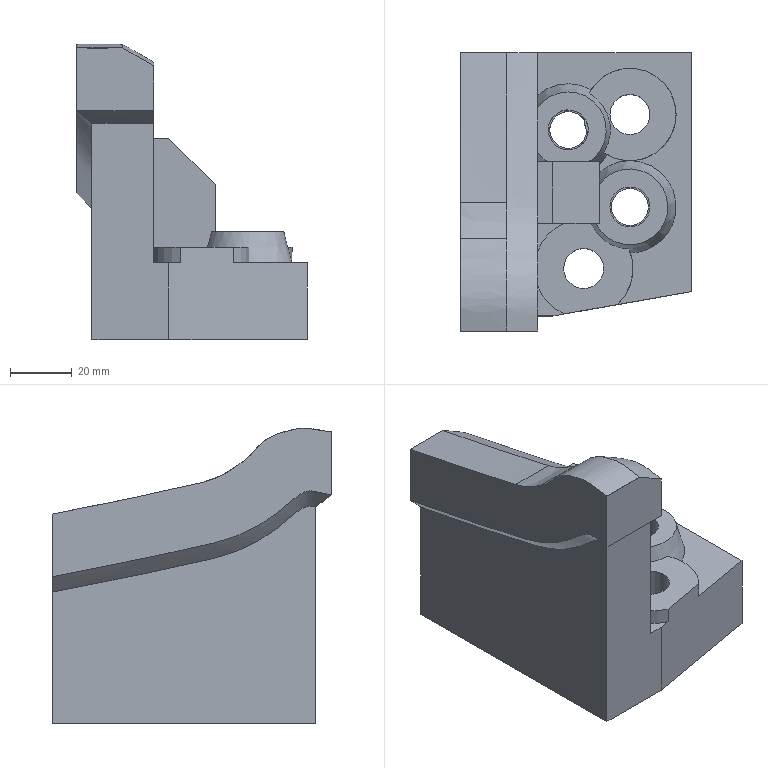Part | NX | features solid 2 | 1 solid | 47 faces | box 75 x 90.482 x 95.908 mm | volume 263627 mm3 | plane 24 | cylinder 11 | spline 9 | cone 3 | commonest cylinder face diameters 13 x4 32 x3 12 x2 30 x2